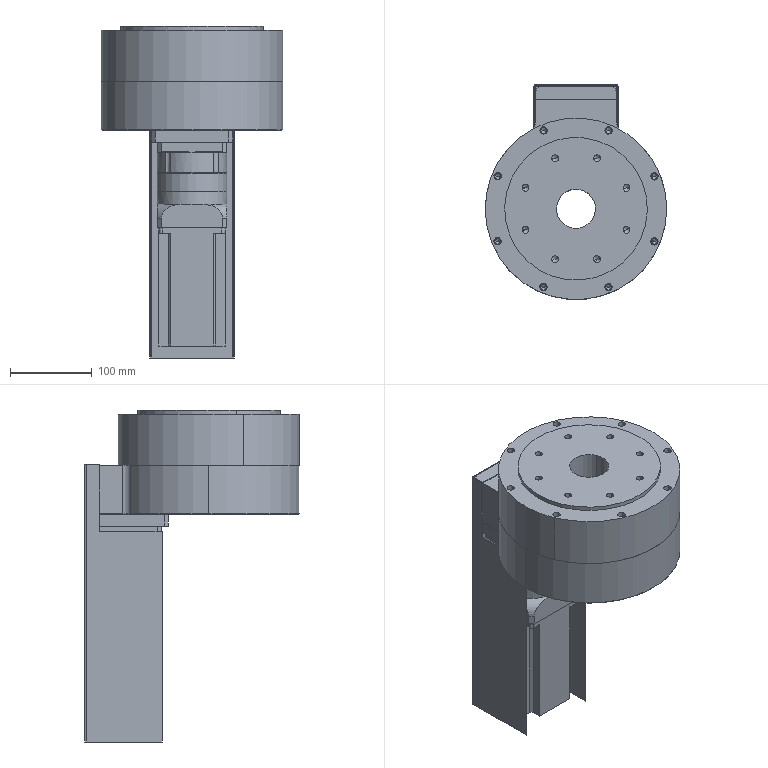Part | SolidWorks | features InContextFeatHolder 12 | 9 solids | 693 faces | box 222.5 x 263.631 x 407 mm | volume 6113754 mm3 | cylinder 390 | plane 168 | cone 114 | torus 13 | spline 8 | commonest cylinder face diameters 17.6 x48 5 x38 6.8 x32 48 x25 38.998 x22 9 x21